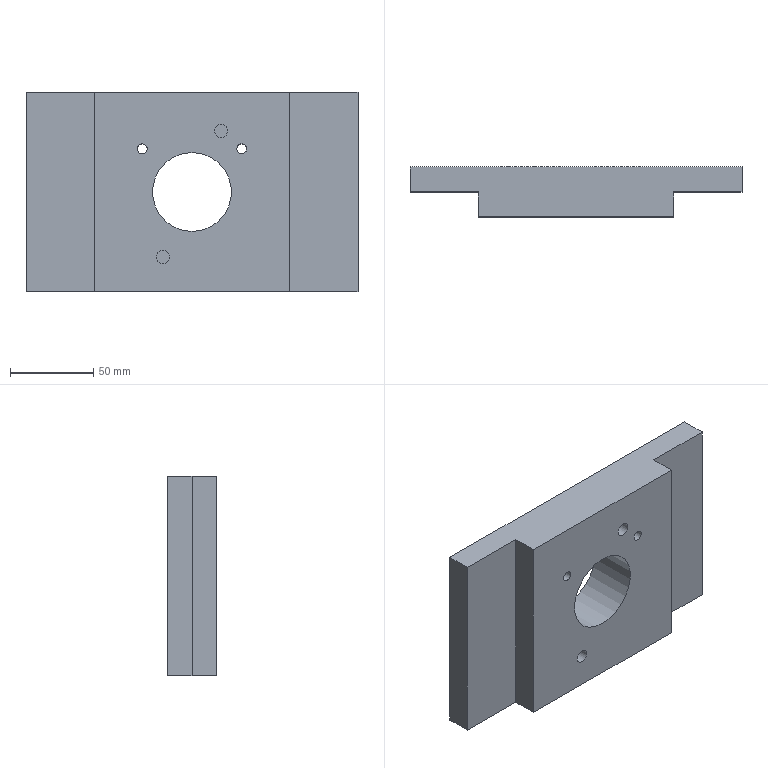Part | NX | features DATUM_CSYS 10, EXTRUDE 10, SKETCH 10, OFFSET_REGION 5, BREP 1, DELETE FACE 1 | 1 solid | 21 faces | box 200 x 30 x 120 mm | volume 506738 mm3 | plane 14 | cylinder 7 | commonest cylinder face diameters 6 x2 8 x2 10 x2 47.518 x1
STEP:
#1=CARTESIAN_POINT('',(-100.,40.,15.));
#2=VERTEX_POINT('',#1);
#3=CARTESIAN_POINT('',(-100.,55.,15.));
#4=VERTEX_POINT('',#3);
#5=CARTESIAN_POINT('',(-100.,-4.563,15.));
#6=DIRECTION('',(0.,1.,0.));
#7=VECTOR('',#6,1000.);
#8=LINE('',#5,#7);
#9=EDGE_CURVE('',#2,#4,#8,.T.);
#10=ORIENTED_EDGE('',*,*,#9,.F.);
#11=CARTESIAN_POINT('',(-100.,40.,135.));
#12=VERTEX_POINT('',#11);
#13=CARTESIAN_POINT('',(-100.,40.,135.));
#14=DIRECTION('',(0.,0.,-1.));
#15=VECTOR('',#14,1000.);
#16=LINE('',#13,#15);
#17=EDGE_CURVE('',#12,#2,#16,.T.);
#18=ORIENTED_EDGE('',*,*,#17,.F.);
#19=CARTESIAN_POINT('',(-100.,55.,135.));
#20=VERTEX_POINT('',#19);
#21=CARTESIAN_POINT('',(-100.,55.,135.));
#22=DIRECTION('',(0.,-1.,0.));
#23=VECTOR('',#22,1000.);
#24=LINE('',#21,#23);
#25=EDGE_CURVE('',#20,#12,#24,.T.);
#26=ORIENTED_EDGE('',*,*,#25,.F.);
#27=CARTESIAN_POINT('',(-100.,55.,135.));
#28=DIRECTION('',(0.,0.,-1.));
#29=VECTOR('',#28,1000.);
#30=LINE('',#27,#29);
#31=EDGE_CURVE('',#20,#4,#30,.T.);
#32=ORIENTED_EDGE('',*,*,#31,.T.);
#33=EDGE_LOOP('',(#10,#18,#26,#32));
#34=FACE_BOUND('',#33,.T.);
#35=CARTESIAN_POINT('',(-100.,75.,15.));
#36=DIRECTION('',(1.,0.,0.));
#37=DIRECTION('',(0.,-1.,0.));
#38=AXIS2_PLACEMENT_3D('',#35,#36,#37);
#39=PLANE('',#38);
#40=ADVANCED_FACE('',(#34),#39,.F.);
#41=CARTESIAN_POINT('',(100.,40.,135.));
#42=VERTEX_POINT('',#41);
#43=CARTESIAN_POINT('',(100.,40.,15.));
#44=VERTEX_POINT('',#43);
#45=CARTESIAN_POINT('',(100.,40.,135.));
#46=DIRECTION('',(0.,0.,-1.));
#47=VECTOR('',#46,1000.);
#48=LINE('',#45,#47);
#49=EDGE_CURVE('',#42,#44,#48,.T.);
#50=ORIENTED_EDGE('',*,*,#49,.T.);
#51=CARTESIAN_POINT('',(100.,55.,15.));
#52=VERTEX_POINT('',#51);
#53=CARTESIAN_POINT('',(100.,75.,15.));
#54=DIRECTION('',(0.,1.,0.));
#55=VECTOR('',#54,1000.);
#56=LINE('',#53,#55);
#57=EDGE_CURVE('',#44,#52,#56,.T.);
#58=ORIENTED_EDGE('',*,*,#57,.T.);
#59=CARTESIAN_POINT('',(100.,55.,135.));
#60=VERTEX_POINT('',#59);
#61=CARTESIAN_POINT('',(100.,55.,135.));
#62=DIRECTION('',(0.,0.,-1.));
#63=VECTOR('',#62,1000.);
#64=LINE('',#61,#63);
#65=EDGE_CURVE('',#60,#52,#64,.T.);
#66=ORIENTED_EDGE('',*,*,#65,.F.);
#67=CARTESIAN_POINT('',(100.,40.,135.));
#68=DIRECTION('',(0.,1.,0.));
#69=VECTOR('',#68,1000.);
#70=LINE('',#67,#69);
#71=EDGE_CURVE('',#42,#60,#70,.T.);
#72=ORIENTED_EDGE('',*,*,#71,.F.);
#73=EDGE_LOOP('',(#50,#58,#66,#72));
#74=FACE_BOUND('',#73,.T.);
#75=CARTESIAN_POINT('',(100.,75.,15.));
#76=DIRECTION('',(-1.,0.,0.));
#77=DIRECTION('',(0.,1.,0.));
#78=AXIS2_PLACEMENT_3D('',#75,#76,#77);
#79=PLANE('',#78);
#80=ADVANCED_FACE('',(#74),#79,.F.);
#81=CARTESIAN_POINT('',(0.,25.,51.241));
#82=VERTEX_POINT('',#81);
#83=CARTESIAN_POINT('',(0.,25.,75.));
#84=DIRECTION('',(0.,-1.,0.));
#85=DIRECTION('',(0.,0.,-1.));
#86=AXIS2_PLACEMENT_3D('',#83,#84,#85);
#87=CIRCLE('',#86,23.759);
#88=EDGE_CURVE('',#82,#82,#87,.F.);
#89=ORIENTED_EDGE('',*,*,#88,.T.);
#90=EDGE_LOOP('',(#89));
#91=FACE_BOUND('',#90,.T.);
#92=CARTESIAN_POINT('',(58.75,25.,15.));
#93=VERTEX_POINT('',#92);
#94=CARTESIAN_POINT('',(-58.75,25.,15.));
#95=VERTEX_POINT('',#94);
#96=CARTESIAN_POINT('',(18.75,25.,15.));
#97=DIRECTION('',(-1.,0.,0.));
#98=VECTOR('',#97,1000.);
#99=LINE('',#96,#98);
#100=EDGE_CURVE('',#93,#95,#99,.T.);
#101=ORIENTED_EDGE('',*,*,#100,.F.);
#102=CARTESIAN_POINT('',(58.75,25.,135.));
#103=VERTEX_POINT('',#102);
#104=CARTESIAN_POINT('',(58.75,25.,15.));
#105=DIRECTION('',(0.,0.,1.));
#106=VECTOR('',#105,1000.);
#107=LINE('',#104,#106);
#108=EDGE_CURVE('',#93,#103,#107,.T.);
#109=ORIENTED_EDGE('',*,*,#108,.T.);
#110=CARTESIAN_POINT('',(-58.75,25.,135.));
#111=VERTEX_POINT('',#110);
#112=CARTESIAN_POINT('',(18.75,25.,135.));
#113=DIRECTION('',(1.,0.,0.));
#114=VECTOR('',#113,1000.);
#115=LINE('',#112,#114);
#116=EDGE_CURVE('',#111,#103,#115,.T.);
#117=ORIENTED_EDGE('',*,*,#116,.F.);
#118=CARTESIAN_POINT('',(-58.75,25.,15.));
#119=DIRECTION('',(0.,0.,1.));
#120=VECTOR('',#119,1000.);
#121=LINE('',#118,#120);
#122=EDGE_CURVE('',#95,#111,#121,.T.);
#123=ORIENTED_EDGE('',*,*,#122,.F.);
#124=EDGE_LOOP('',(#101,#109,#117,#123));
#125=FACE_BOUND('',#124,.T.);
#126=CARTESIAN_POINT('',(-27.,25.,101.));
#127=VERTEX_POINT('',#126);
#128=CARTESIAN_POINT('',(-30.,25.,101.));
#129=DIRECTION('',(0.,-1.,0.));
#130=DIRECTION('',(1.,0.,0.));
#131=AXIS2_PLACEMENT_3D('',#128,#129,#130);
#132=CIRCLE('',#131,3.);
#133=EDGE_CURVE('',#127,#127,#132,.T.);
#134=ORIENTED_EDGE('',*,*,#133,.F.);
#135=EDGE_LOOP('',(#134));
#136=FACE_BOUND('',#135,.T.);
#137=CARTESIAN_POINT('',(33.,25.,101.));
#138=VERTEX_POINT('',#137);
#139=CARTESIAN_POINT('',(30.,25.,101.));
#140=DIRECTION('',(0.,-1.,0.));
#141=DIRECTION('',(1.,0.,0.));
#142=AXIS2_PLACEMENT_3D('',#139,#140,#141);
#143=CIRCLE('',#142,3.);
#144=EDGE_CURVE('',#138,#138,#143,.T.);
#145=ORIENTED_EDGE('',*,*,#144,.F.);
#146=EDGE_LOOP('',(#145));
#147=FACE_BOUND('',#146,.T.);
#148=CARTESIAN_POINT('',(21.5,25.,111.832));
#149=VERTEX_POINT('',#148);
#150=CARTESIAN_POINT('',(17.5,25.,111.832));
#151=DIRECTION('',(0.,-1.,0.));
#152=DIRECTION('',(1.,0.,0.));
#153=AXIS2_PLACEMENT_3D('',#150,#151,#152);
#154=CIRCLE('',#153,4.);
#155=EDGE_CURVE('',#149,#149,#154,.T.);
#156=ORIENTED_EDGE('',*,*,#155,.F.);
#157=EDGE_LOOP('',(#156));
#158=FACE_BOUND('',#157,.T.);
#159=CARTESIAN_POINT('',(-13.5,25.,35.832));
#160=VERTEX_POINT('',#159);
#161=CARTESIAN_POINT('',(-17.5,25.,35.832));
#162=DIRECTION('',(0.,-1.,0.));
#163=DIRECTION('',(1.,0.,0.));
#164=AXIS2_PLACEMENT_3D('',#161,#162,#163);
#165=CIRCLE('',#164,4.);
#166=EDGE_CURVE('',#160,#160,#165,.F.);
#167=ORIENTED_EDGE('',*,*,#166,.T.);
#168=EDGE_LOOP('',(#167));
#169=FACE_BOUND('',#168,.T.);
#170=CARTESIAN_POINT('',(18.75,25.,15.));
#171=DIRECTION('',(0.,-1.,0.));
#172=DIRECTION('',(0.,0.,1.));
#173=AXIS2_PLACEMENT_3D('',#170,#171,#172);
#174=PLANE('',#173);
#175=ADVANCED_FACE('',(#91,#125,#136,#147,#158,#169),#174,.T.);
#176=ORIENTED_EDGE('',*,*,#17,.T.);
#177=CARTESIAN_POINT('',(-58.75,40.,15.));
#178=VERTEX_POINT('',#177);
#179=CARTESIAN_POINT('',(100.,40.,15.));
#180=DIRECTION('',(1.,0.,0.));
#181=VECTOR('',#180,1000.);
#182=LINE('',#179,#181);
#183=EDGE_CURVE('',#2,#178,#182,.T.);
#184=ORIENTED_EDGE('',*,*,#183,.T.);
#185=CARTESIAN_POINT('',(-58.75,40.,135.));
#186=VERTEX_POINT('',#185);
#187=CARTESIAN_POINT('',(-58.75,40.,15.));
#188=DIRECTION('',(0.,0.,1.));
#189=VECTOR('',#188,1000.);
#190=LINE('',#187,#189);
#191=EDGE_CURVE('',#178,#186,#190,.T.);
#192=ORIENTED_EDGE('',*,*,#191,.T.);
#193=CARTESIAN_POINT('',(100.,40.,135.));
#194=DIRECTION('',(1.,0.,0.));
#195=VECTOR('',#194,1000.);
#196=LINE('',#193,#195);
#197=EDGE_CURVE('',#12,#186,#196,.T.);
#198=ORIENTED_EDGE('',*,*,#197,.F.);
#199=EDGE_LOOP('',(#176,#184,#192,#198));
#200=FACE_BOUND('',#199,.T.);
#201=CARTESIAN_POINT('',(100.,40.,135.));
#202=DIRECTION('',(0.,1.,0.));
#203=DIRECTION('',(1.,0.,0.));
#204=AXIS2_PLACEMENT_3D('',#201,#202,#203);
#205=PLANE('',#204);
#206=ADVANCED_FACE('',(#200),#205,.F.);
#207=CARTESIAN_POINT('',(0.,55.,98.759));
#208=VERTEX_POINT('',#207);
#209=CARTESIAN_POINT('',(0.,55.,75.));
#210=DIRECTION('',(0.,-1.,0.));
#211=DIRECTION('',(0.,0.,1.));
#212=AXIS2_PLACEMENT_3D('',#209,#210,#211);
#213=CIRCLE('',#212,23.759);
#214=EDGE_CURVE('',#208,#208,#213,.T.);
#215=ORIENTED_EDGE('',*,*,#214,.T.);
#216=EDGE_LOOP('',(#215));
#217=FACE_BOUND('',#216,.T.);
#218=ORIENTED_EDGE('',*,*,#65,.T.);
#219=CARTESIAN_POINT('',(180.,55.,15.));
#220=DIRECTION('',(-1.,0.,0.));
#221=VECTOR('',#220,1000.);
#222=LINE('',#219,#221);
#223=EDGE_CURVE('',#52,#4,#222,.T.);
#224=ORIENTED_EDGE('',*,*,#223,.T.);
#225=ORIENTED_EDGE('',*,*,#31,.F.);
#226=CARTESIAN_POINT('',(100.,55.,135.));
#227=DIRECTION('',(-1.,0.,0.));
#228=VECTOR('',#227,1000.);
#229=LINE('',#226,#228);
#230=EDGE_CURVE('',#60,#20,#229,.T.);
#231=ORIENTED_EDGE('',*,*,#230,.F.);
#232=EDGE_LOOP('',(#218,#224,#225,#231));
#233=FACE_BOUND('',#232,.T.);
#234=CARTESIAN_POINT('',(-30.,55.,98.));
#235=VERTEX_POINT('',#234);
#236=CARTESIAN_POINT('',(-30.,55.,101.));
#237=DIRECTION('',(0.,-1.,0.));
#238=DIRECTION('',(0.,0.,-1.));
#239=AXIS2_PLACEMENT_3D('',#236,#237,#238);
#240=CIRCLE('',#239,3.);
#241=EDGE_CURVE('',#235,#235,#240,.F.);
#242=ORIENTED_EDGE('',*,*,#241,.F.);
#243=EDGE_LOOP('',(#242));
#244=FACE_BOUND('',#243,.T.);
#245=CARTESIAN_POINT('',(30.,55.,98.));
#246=VERTEX_POINT('',#245);
#247=CARTESIAN_POINT('',(30.,55.,101.));
#248=DIRECTION('',(0.,-1.,0.));
#249=DIRECTION('',(0.,0.,-1.));
#250=AXIS2_PLACEMENT_3D('',#247,#248,#249);
#251=CIRCLE('',#250,3.);
#252=EDGE_CURVE('',#246,#246,#251,.F.);
#253=ORIENTED_EDGE('',*,*,#252,.F.);
#254=EDGE_LOOP('',(#253));
#255=FACE_BOUND('',#254,.T.);
#256=CARTESIAN_POINT('',(100.,55.,135.));
#257=DIRECTION('',(0.,-1.,0.));
#258=DIRECTION('',(0.,0.,1.));
#259=AXIS2_PLACEMENT_3D('',#256,#257,#258);
#260=PLANE('',#259);
#261=ADVANCED_FACE('',(#217,#233,#244,#255),#260,.F.);
#262=CARTESIAN_POINT('',(58.75,40.,15.));
#263=VERTEX_POINT('',#262);
#264=CARTESIAN_POINT('',(58.75,40.,135.));
#265=VERTEX_POINT('',#264);
#266=CARTESIAN_POINT('',(58.75,40.,135.));
#267=DIRECTION('',(0.,0.,1.));
#268=VECTOR('',#267,1000.);
#269=LINE('',#266,#268);
#270=EDGE_CURVE('',#263,#265,#269,.T.);
#271=ORIENTED_EDGE('',*,*,#270,.F.);
#272=CARTESIAN_POINT('',(100.,40.,15.));
#273=DIRECTION('',(1.,0.,0.));
#274=VECTOR('',#273,1000.);
#275=LINE('',#272,#274);
#276=EDGE_CURVE('',#263,#44,#275,.T.);
#277=ORIENTED_EDGE('',*,*,#276,.T.);
#278=ORIENTED_EDGE('',*,*,#49,.F.);
#279=CARTESIAN_POINT('',(100.,40.,135.));
#280=DIRECTION('',(1.,0.,0.));
#281=VECTOR('',#280,1000.);
#282=LINE('',#279,#281);
#283=EDGE_CURVE('',#265,#42,#282,.T.);
#284=ORIENTED_EDGE('',*,*,#283,.F.);
#285=EDGE_LOOP('',(#271,#277,#278,#284));
#286=FACE_BOUND('',#285,.T.);
#287=CARTESIAN_POINT('',(100.,40.,135.));
#288=DIRECTION('',(0.,1.,0.));
#289=DIRECTION('',(1.,0.,0.));
#290=AXIS2_PLACEMENT_3D('',#287,#288,#289);
#291=PLANE('',#290);
#292=ADVANCED_FACE('',(#286),#291,.F.);
#293=CARTESIAN_POINT('',(58.75,0.,135.));
#294=DIRECTION('',(0.,-1.,0.));
#295=VECTOR('',#294,1000.);
#296=LINE('',#293,#295);
#297=EDGE_CURVE('',#265,#103,#296,.T.);
#298=ORIENTED_EDGE('',*,*,#297,.F.);
#299=ORIENTED_EDGE('',*,*,#283,.T.);
#300=ORIENTED_EDGE('',*,*,#71,.T.);
#301=ORIENTED_EDGE('',*,*,#230,.T.);
#302=ORIENTED_EDGE('',*,*,#25,.T.);
#303=ORIENTED_EDGE('',*,*,#197,.T.);
#304=CARTESIAN_POINT('',(-58.75,0.,135.));
#305=DIRECTION('',(0.,1.,0.));
#306=VECTOR('',#305,1000.);
#307=LINE('',#304,#306);
#308=EDGE_CURVE('',#111,#186,#307,.T.);
#309=ORIENTED_EDGE('',*,*,#308,.F.);
#310=ORIENTED_EDGE('',*,*,#116,.T.);
#311=EDGE_LOOP('',(#298,#299,#300,#301,#302,#303,#309,#310));
#312=FACE_BOUND('',#311,.T.);
#313=CARTESIAN_POINT('',(0.,0.,135.));
#314=DIRECTION('',(0.,0.,1.));
#315=DIRECTION('',(-1.,0.,0.));
#316=AXIS2_PLACEMENT_3D('',#313,#314,#315);
#317=PLANE('',#316);
#318=ADVANCED_FACE('',(#312),#317,.T.);
#319=ORIENTED_EDGE('',*,*,#191,.F.);
#320=CARTESIAN_POINT('',(-58.75,25.,15.));
#321=DIRECTION('',(0.,-1.,0.));
#322=VECTOR('',#321,1000.);
#323=LINE('',#320,#322);
#324=EDGE_CURVE('',#178,#95,#323,.T.);
#325=ORIENTED_EDGE('',*,*,#324,.T.);
#326=ORIENTED_EDGE('',*,*,#122,.T.);
#327=ORIENTED_EDGE('',*,*,#308,.T.);
#328=EDGE_LOOP('',(#319,#325,#326,#327));
#329=FACE_BOUND('',#328,.T.);
#330=CARTESIAN_POINT('',(-58.75,25.,15.));
#331=DIRECTION('',(1.,0.,0.));
#332=DIRECTION('',(0.,0.,-1.));
#333=AXIS2_PLACEMENT_3D('',#330,#331,#332);
#334=PLANE('',#333);
#335=ADVANCED_FACE('',(#329),#334,.F.);
#336=ORIENTED_EDGE('',*,*,#108,.F.);
#337=CARTESIAN_POINT('',(58.75,40.,15.));
#338=DIRECTION('',(0.,1.,0.));
#339=VECTOR('',#338,1000.);
#340=LINE('',#337,#339);
#341=EDGE_CURVE('',#93,#263,#340,.T.);
#342=ORIENTED_EDGE('',*,*,#341,.T.);
#343=ORIENTED_EDGE('',*,*,#270,.T.);
#344=ORIENTED_EDGE('',*,*,#297,.T.);
#345=EDGE_LOOP('',(#336,#342,#343,#344));
#346=FACE_BOUND('',#345,.T.);
#347=CARTESIAN_POINT('',(58.75,40.,15.));
#348=DIRECTION('',(-1.,0.,0.));
#349=DIRECTION('',(0.,0.,1.));
#350=AXIS2_PLACEMENT_3D('',#347,#348,#349);
#351=PLANE('',#350);
#352=ADVANCED_FACE('',(#346),#351,.F.);
#353=CARTESIAN_POINT('',(21.5,45.,111.832));
#354=VERTEX_POINT('',#353);
#355=CARTESIAN_POINT('',(17.5,45.,111.832));
#356=DIRECTION('',(0.,-1.,0.));
#357=DIRECTION('',(1.,0.,0.));
#358=AXIS2_PLACEMENT_3D('',#355,#356,#357);
#359=CIRCLE('',#358,4.);
#360=EDGE_CURVE('',#354,#354,#359,.F.);
#361=ORIENTED_EDGE('',*,*,#360,.T.);
#362=EDGE_LOOP('',(#361));
#363=FACE_BOUND('',#362,.T.);
#364=ORIENTED_EDGE('',*,*,#155,.T.);
#365=EDGE_LOOP('',(#364));
#366=FACE_BOUND('',#365,.T.);
#367=CARTESIAN_POINT('',(17.5,45.,111.832));
#368=DIRECTION('',(0.,-1.,0.));
#369=DIRECTION('',(0.,0.,-1.));
#370=AXIS2_PLACEMENT_3D('',#367,#368,#369);
#371=CYLINDRICAL_SURFACE('',#370,4.);
#372=ADVANCED_FACE('',(#363,#366),#371,.F.);
#373=ORIENTED_EDGE('',*,*,#360,.F.);
#374=EDGE_LOOP('',(#373));
#375=FACE_BOUND('',#374,.T.);
#376=CARTESIAN_POINT('',(17.5,45.,111.832));
#377=DIRECTION('',(0.,-1.,0.));
#378=DIRECTION('',(0.,0.,-1.));
#379=AXIS2_PLACEMENT_3D('',#376,#377,#378);
#380=PLANE('',#379);
#381=ADVANCED_FACE('',(#375),#380,.T.);
#382=CARTESIAN_POINT('',(-13.5,45.,35.832));
#383=VERTEX_POINT('',#382);
#384=CARTESIAN_POINT('',(-17.5,45.,35.832));
#385=DIRECTION('',(0.,-1.,0.));
#386=DIRECTION('',(1.,0.,0.));
#387=AXIS2_PLACEMENT_3D('',#384,#385,#386);
#388=CIRCLE('',#387,4.);
#389=EDGE_CURVE('',#383,#383,#388,.T.);
#390=ORIENTED_EDGE('',*,*,#389,.F.);
#391=EDGE_LOOP('',(#390));
#392=FACE_BOUND('',#391,.T.);
#393=ORIENTED_EDGE('',*,*,#166,.F.);
#394=EDGE_LOOP('',(#393));
#395=FACE_BOUND('',#394,.T.);
#396=CARTESIAN_POINT('',(-17.5,45.,35.832));
#397=DIRECTION('',(0.,-1.,0.));
#398=DIRECTION('',(0.,0.,-1.));
#399=AXIS2_PLACEMENT_3D('',#396,#397,#398);
#400=CYLINDRICAL_SURFACE('',#399,4.);
#401=ADVANCED_FACE('',(#392,#395),#400,.F.);
#402=ORIENTED_EDGE('',*,*,#389,.T.);
#403=EDGE_LOOP('',(#402));
#404=FACE_BOUND('',#403,.T.);
#405=CARTESIAN_POINT('',(-17.5,45.,35.832));
#406=DIRECTION('',(0.,-1.,0.));
#407=DIRECTION('',(0.,0.,-1.));
#408=AXIS2_PLACEMENT_3D('',#405,#406,#407);
#409=PLANE('',#408);
#410=ADVANCED_FACE('',(#404),#409,.T.);
#411=ORIENTED_EDGE('',*,*,#252,.T.);
#412=EDGE_LOOP('',(#411));
#413=FACE_BOUND('',#412,.T.);
#414=ORIENTED_EDGE('',*,*,#144,.T.);
#415=EDGE_LOOP('',(#414));
#416=FACE_BOUND('',#415,.T.);
#417=CARTESIAN_POINT('',(30.,55025.,101.));
#418=DIRECTION('',(0.,-1.,0.));
#419=DIRECTION('',(0.,0.,-1.));
#420=AXIS2_PLACEMENT_3D('',#417,#418,#419);
#421=CYLINDRICAL_SURFACE('',#420,3.);
#422=ADVANCED_FACE('',(#413,#416),#421,.F.);
#423=ORIENTED_EDGE('',*,*,#241,.T.);
#424=EDGE_LOOP('',(#423));
#425=FACE_BOUND('',#424,.T.);
#426=ORIENTED_EDGE('',*,*,#133,.T.);
#427=EDGE_LOOP('',(#426));
#428=FACE_BOUND('',#427,.T.);
#429=CARTESIAN_POINT('',(-30.,55025.,101.));
#430=DIRECTION('',(0.,-1.,0.));
#431=DIRECTION('',(0.,0.,-1.));
#432=AXIS2_PLACEMENT_3D('',#429,#430,#431);
#433=CYLINDRICAL_SURFACE('',#432,3.);
#434=ADVANCED_FACE('',(#425,#428),#433,.F.);
#435=CARTESIAN_POINT('',(-85.,47.5,15.));
#436=VERTEX_POINT('',#435);
#437=CARTESIAN_POINT('',(-80.,47.5,15.));
#438=DIRECTION('',(0.,0.,-1.));
#439=DIRECTION('',(-1.,0.,0.));
#440=AXIS2_PLACEMENT_3D('',#437,#438,#439);
#441=CIRCLE('',#440,5.);
#442=EDGE_CURVE('',#436,#436,#441,.T.);
#443=ORIENTED_EDGE('',*,*,#442,.F.);
#444=EDGE_LOOP('',(#443));
#445=FACE_BOUND('',#444,.T.);
#446=CARTESIAN_POINT('',(75.,47.5,15.));
#447=VERTEX_POINT('',#446);
#448=CARTESIAN_POINT('',(80.,47.5,15.));
#449=DIRECTION('',(0.,0.,-1.));
#450=DIRECTION('',(-1.,0.,0.));
#451=AXIS2_PLACEMENT_3D('',#448,#449,#450);
#452=CIRCLE('',#451,5.);
#453=EDGE_CURVE('',#447,#447,#452,.T.);
#454=ORIENTED_EDGE('',*,*,#453,.F.);
#455=EDGE_LOOP('',(#454));
#456=FACE_BOUND('',#455,.T.);
#457=ORIENTED_EDGE('',*,*,#9,.T.);
#458=ORIENTED_EDGE('',*,*,#223,.F.);
#459=ORIENTED_EDGE('',*,*,#57,.F.);
#460=ORIENTED_EDGE('',*,*,#276,.F.);
#461=ORIENTED_EDGE('',*,*,#341,.F.);
#462=ORIENTED_EDGE('',*,*,#100,.T.);
#463=ORIENTED_EDGE('',*,*,#324,.F.);
#464=ORIENTED_EDGE('',*,*,#183,.F.);
#465=EDGE_LOOP('',(#457,#458,#459,#460,#461,#462,#463,#464));
#466=FACE_BOUND('',#465,.T.);
#467=CARTESIAN_POINT('',(180.,-4.563,15.));
#468=DIRECTION('',(0.,0.,1.));
#469=DIRECTION('',(0.,-1.,0.));
#470=AXIS2_PLACEMENT_3D('',#467,#468,#469);
#471=PLANE('',#470);
#472=ADVANCED_FACE('',(#445,#456,#466),#471,.F.);
#473=ORIENTED_EDGE('',*,*,#453,.T.);
#474=EDGE_LOOP('',(#473));
#475=FACE_BOUND('',#474,.T.);
#476=CARTESIAN_POINT('',(75.,47.5,65.));
#477=VERTEX_POINT('',#476);
#478=CARTESIAN_POINT('',(80.,47.5,65.));
#479=DIRECTION('',(0.,0.,-1.));
#480=DIRECTION('',(-1.,0.,0.));
#481=AXIS2_PLACEMENT_3D('',#478,#479,#480);
#482=CIRCLE('',#481,5.);
#483=EDGE_CURVE('',#477,#477,#482,.T.);
#484=ORIENTED_EDGE('',*,*,#483,.F.);
#485=EDGE_LOOP('',(#484));
#486=FACE_BOUND('',#485,.T.);
#487=CARTESIAN_POINT('',(80.,47.5,30.));
#488=DIRECTION('',(0.,0.,-1.));
#489=DIRECTION('',(0.,1.,0.));
#490=AXIS2_PLACEMENT_3D('',#487,#488,#489);
#491=CYLINDRICAL_SURFACE('',#490,5.);
#492=ADVANCED_FACE('',(#475,#486),#491,.F.);
#493=ORIENTED_EDGE('',*,*,#442,.T.);
#494=EDGE_LOOP('',(#493));
#495=FACE_BOUND('',#494,.T.);
#496=CARTESIAN_POINT('',(-85.,47.5,65.));
#497=VERTEX_POINT('',#496);
#498=CARTESIAN_POINT('',(-80.,47.5,65.));
#499=DIRECTION('',(0.,0.,-1.));
#500=DIRECTION('',(-1.,0.,0.));
#501=AXIS2_PLACEMENT_3D('',#498,#499,#500);
#502=CIRCLE('',#501,5.);
#503=EDGE_CURVE('',#497,#497,#502,.T.);
#504=ORIENTED_EDGE('',*,*,#503,.F.);
#505=EDGE_LOOP('',(#504));
#506=FACE_BOUND('',#505,.T.);
#507=CARTESIAN_POINT('',(-80.,47.5,30.));
#508=DIRECTION('',(0.,0.,-1.));
#509=DIRECTION('',(0.,1.,0.));
#510=AXIS2_PLACEMENT_3D('',#507,#508,#509);
#511=CYLINDRICAL_SURFACE('',#510,5.);
#512=ADVANCED_FACE('',(#495,#506),#511,.F.);
#513=ORIENTED_EDGE('',*,*,#88,.F.);
#514=EDGE_LOOP('',(#513));
#515=FACE_BOUND('',#514,.T.);
#516=ORIENTED_EDGE('',*,*,#214,.F.);
#517=EDGE_LOOP('',(#516));
#518=FACE_BOUND('',#517,.T.);
#519=CARTESIAN_POINT('',(0.,-95.,75.));
#520=DIRECTION('',(0.,1.,0.));
#521=DIRECTION('',(0.,0.,1.));
#522=AXIS2_PLACEMENT_3D('',#519,#520,#521);
#523=CYLINDRICAL_SURFACE('',#522,23.759);
#524=ADVANCED_FACE('',(#515,#518),#523,.F.);
#525=ORIENTED_EDGE('',*,*,#503,.T.);
#526=EDGE_LOOP('',(#525));
#527=FACE_BOUND('',#526,.T.);
#528=CARTESIAN_POINT('',(-80.,47.5,65.));
#529=DIRECTION('',(0.,0.,-1.));
#530=DIRECTION('',(0.,1.,0.));
#531=AXIS2_PLACEMENT_3D('',#528,#529,#530);
#532=PLANE('',#531);
#533=ADVANCED_FACE('',(#527),#532,.T.);
#534=ORIENTED_EDGE('',*,*,#483,.T.);
#535=EDGE_LOOP('',(#534));
#536=FACE_BOUND('',#535,.T.);
#537=CARTESIAN_POINT('',(80.,47.5,65.));
#538=DIRECTION('',(0.,0.,-1.));
#539=DIRECTION('',(0.,1.,0.));
#540=AXIS2_PLACEMENT_3D('',#537,#538,#539);
#541=PLANE('',#540);
#542=ADVANCED_FACE('',(#536),#541,.T.);
#543=CLOSED_SHELL('',(#40,#80,#175,#206,#261,#292,#318,#335,#352,#372,#381,#401,#410,#422,#434,#472,#492,#512,#524,#533,#542));
#544=MANIFOLD_SOLID_BREP('',#543);
#545=(LENGTH_UNIT()NAMED_UNIT(*)SI_UNIT(.MILLI.,.METRE.));
#546=UNCERTAINTY_MEASURE_WITH_UNIT(LENGTH_MEASURE(0.00001),#545,'','');
#547=(NAMED_UNIT(*)PLANE_ANGLE_UNIT()SI_UNIT($,.RADIAN.));
#548=(NAMED_UNIT(*)SI_UNIT($,.STERADIAN.)SOLID_ANGLE_UNIT());
#549=(GEOMETRIC_REPRESENTATION_CONTEXT(3)GLOBAL_UNCERTAINTY_ASSIGNED_CONTEXT((#546))GLOBAL_UNIT_ASSIGNED_CONTEXT((#545,#547,#548))REPRESENTATION_CONTEXT('',''));
#550=ADVANCED_BREP_SHAPE_REPRESENTATION('',(#544),#549);